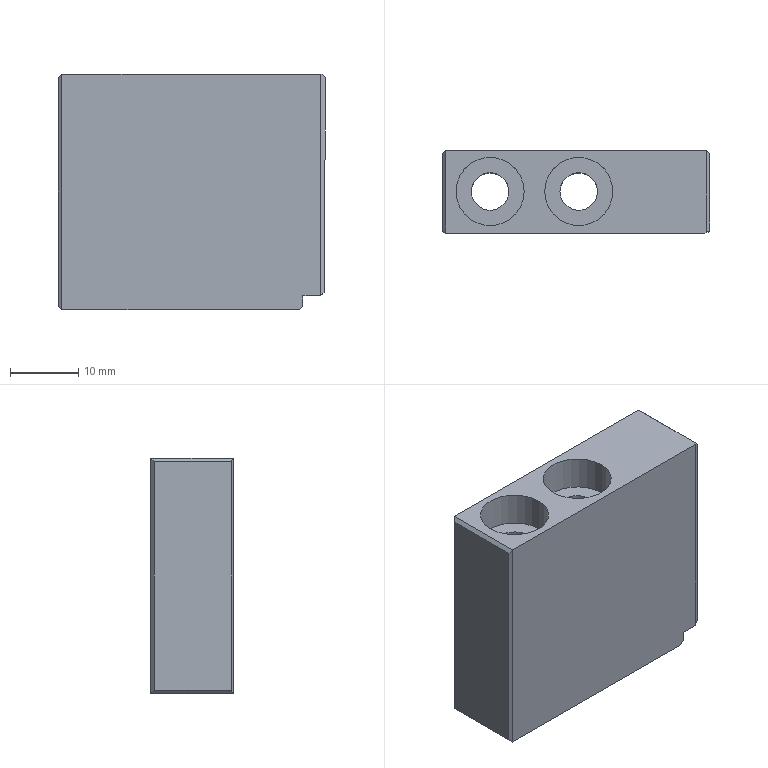Part | STEP file | side block 3 | 1 solid | 27 faces | box 39.196 x 12.1 x 34.5 mm | volume 14030 mm3 | plane 19 | cylinder 8 | commonest cylinder face diameters 5.5 x4 10 x4